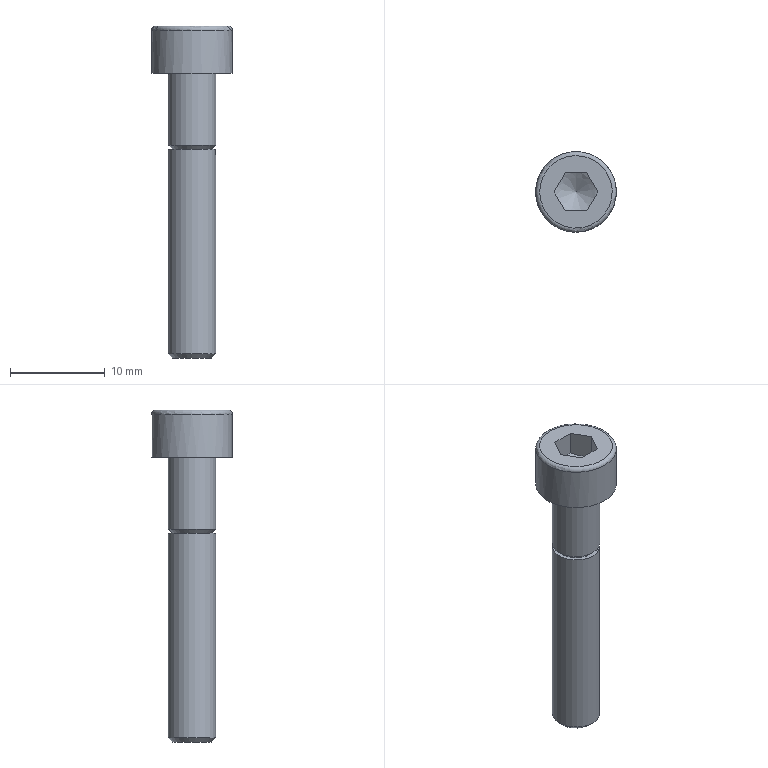Part | STEP file | 1_35 | 1 solid | 17 faces | box 8.5 x 8.5 x 35 mm | volume 827.103 mm3 | plane 10 | cylinder 3 | cone 3 | torus 1 | commonest cylinder face diameters 5 x2 8.5 x1